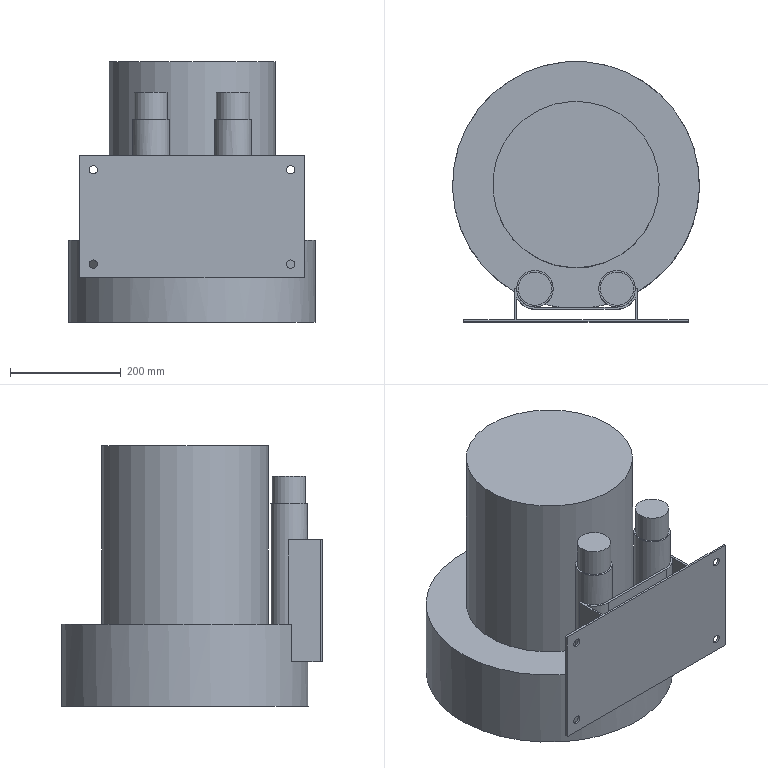Part | STEP file | High-pressure fan RB-81D-2  5.5 | 1 solid | 39 faces | box 445 x 470 x 470 mm | volume 48196616 mm3 | plane 25 | cylinder 14 | commonest cylinder face diameters 15 x4 66 x4 60 x2 74 x2 300 x1 445 x1
STEP:
#1=CARTESIAN_POINT('',(-107.,-187.5,300.));
#2=VERTEX_POINT('',#1);
#3=CARTESIAN_POINT('',(-74.,-220.5,300.));
#4=VERTEX_POINT('',#3);
#5=CARTESIAN_POINT('',(-74.,-187.5,300.));
#6=DIRECTION('',(0.,0.,1.));
#7=DIRECTION('',(-1.,0.,0.));
#8=AXIS2_PLACEMENT_3D('',#5,#6,#7);
#9=CIRCLE('',#8,33.);
#10=EDGE_CURVE('',#2,#4,#9,.T.);
#11=ORIENTED_EDGE('',*,*,#10,.T.);
#12=CARTESIAN_POINT('',(-74.,-220.5,148.));
#13=VERTEX_POINT('',#12);
#14=CARTESIAN_POINT('',(-74.,-220.5,300.));
#15=DIRECTION('',(0.,0.,-1.));
#16=VECTOR('',#15,1000.);
#17=LINE('',#14,#16);
#18=EDGE_CURVE('',#4,#13,#17,.T.);
#19=ORIENTED_EDGE('',*,*,#18,.T.);
#20=CARTESIAN_POINT('',(-56.197,-215.286,148.));
#21=VERTEX_POINT('',#20);
#22=CARTESIAN_POINT('',(-74.,-187.5,148.));
#23=DIRECTION('',(0.,0.,1.));
#24=DIRECTION('',(1.,0.,0.));
#25=AXIS2_PLACEMENT_3D('',#22,#23,#24);
#26=CIRCLE('',#25,33.);
#27=EDGE_CURVE('',#13,#21,#26,.T.);
#28=ORIENTED_EDGE('',*,*,#27,.T.);
#29=CARTESIAN_POINT('',(-107.,-187.5,148.));
#30=VERTEX_POINT('',#29);
#31=CARTESIAN_POINT('',(-74.,-187.5,148.));
#32=DIRECTION('',(0.,0.,-1.));
#33=DIRECTION('',(1.,0.,0.));
#34=AXIS2_PLACEMENT_3D('',#31,#32,#33);
#35=CIRCLE('',#34,33.);
#36=EDGE_CURVE('',#30,#21,#35,.T.);
#37=ORIENTED_EDGE('',*,*,#36,.F.);
#38=CARTESIAN_POINT('',(-107.,-187.5,300.));
#39=DIRECTION('',(0.,0.,-1.));
#40=VECTOR('',#39,1000.);
#41=LINE('',#38,#40);
#42=EDGE_CURVE('',#2,#30,#41,.T.);
#43=ORIENTED_EDGE('',*,*,#42,.F.);
#44=EDGE_LOOP('',(#11,#19,#28,#37,#43));
#45=FACE_OUTER_BOUND('',#44,.T.);
#46=CARTESIAN_POINT('',(-41.,-187.5,365.));
#47=VERTEX_POINT('',#46);
#48=CARTESIAN_POINT('',(-74.,-187.5,365.));
#49=DIRECTION('',(0.,0.,1.));
#50=DIRECTION('',(1.,0.,0.));
#51=AXIS2_PLACEMENT_3D('',#48,#49,#50);
#52=CIRCLE('',#51,33.);
#53=EDGE_CURVE('',#47,#47,#52,.T.);
#54=ORIENTED_EDGE('',*,*,#53,.F.);
#55=EDGE_LOOP('',(#54));
#56=FACE_OUTER_BOUND('',#55,.T.);
#57=CARTESIAN_POINT('',(-74.,-187.5,415.));
#58=DIRECTION('',(0.,0.,-1.));
#59=DIRECTION('',(-1.,0.,0.));
#60=AXIS2_PLACEMENT_3D('',#57,#58,#59);
#61=CYLINDRICAL_SURFACE('',#60,33.);
#62=ADVANCED_FACE('',(#45,#56),#61,.T.);
#63=CARTESIAN_POINT('',(74.,-220.5,300.));
#64=VERTEX_POINT('',#63);
#65=CARTESIAN_POINT('',(107.,-187.5,300.));
#66=VERTEX_POINT('',#65);
#67=CARTESIAN_POINT('',(74.,-187.5,300.));
#68=DIRECTION('',(0.,0.,1.));
#69=DIRECTION('',(-1.,0.,0.));
#70=AXIS2_PLACEMENT_3D('',#67,#68,#69);
#71=CIRCLE('',#70,33.);
#72=EDGE_CURVE('',#64,#66,#71,.T.);
#73=ORIENTED_EDGE('',*,*,#72,.T.);
#74=CARTESIAN_POINT('',(107.,-187.5,148.));
#75=VERTEX_POINT('',#74);
#76=CARTESIAN_POINT('',(107.,-187.5,300.));
#77=DIRECTION('',(0.,0.,-1.));
#78=VECTOR('',#77,1000.);
#79=LINE('',#76,#78);
#80=EDGE_CURVE('',#66,#75,#79,.T.);
#81=ORIENTED_EDGE('',*,*,#80,.T.);
#82=CARTESIAN_POINT('',(56.197,-215.286,148.));
#83=VERTEX_POINT('',#82);
#84=CARTESIAN_POINT('',(74.,-187.5,148.));
#85=DIRECTION('',(0.,0.,-1.));
#86=DIRECTION('',(1.,0.,0.));
#87=AXIS2_PLACEMENT_3D('',#84,#85,#86);
#88=CIRCLE('',#87,33.);
#89=EDGE_CURVE('',#83,#75,#88,.T.);
#90=ORIENTED_EDGE('',*,*,#89,.F.);
#91=CARTESIAN_POINT('',(74.,-220.5,148.));
#92=VERTEX_POINT('',#91);
#93=CARTESIAN_POINT('',(74.,-187.5,148.));
#94=DIRECTION('',(0.,0.,1.));
#95=DIRECTION('',(1.,0.,0.));
#96=AXIS2_PLACEMENT_3D('',#93,#94,#95);
#97=CIRCLE('',#96,33.);
#98=EDGE_CURVE('',#83,#92,#97,.T.);
#99=ORIENTED_EDGE('',*,*,#98,.T.);
#100=CARTESIAN_POINT('',(74.,-220.5,300.));
#101=DIRECTION('',(0.,0.,-1.));
#102=VECTOR('',#101,1000.);
#103=LINE('',#100,#102);
#104=EDGE_CURVE('',#64,#92,#103,.T.);
#105=ORIENTED_EDGE('',*,*,#104,.F.);
#106=EDGE_LOOP('',(#73,#81,#90,#99,#105));
#107=FACE_OUTER_BOUND('',#106,.T.);
#108=CARTESIAN_POINT('',(107.,-187.5,365.));
#109=VERTEX_POINT('',#108);
#110=CARTESIAN_POINT('',(74.,-187.5,365.));
#111=DIRECTION('',(0.,0.,1.));
#112=DIRECTION('',(1.,0.,0.));
#113=AXIS2_PLACEMENT_3D('',#110,#111,#112);
#114=CIRCLE('',#113,33.);
#115=EDGE_CURVE('',#109,#109,#114,.T.);
#116=ORIENTED_EDGE('',*,*,#115,.F.);
#117=EDGE_LOOP('',(#116));
#118=FACE_OUTER_BOUND('',#117,.T.);
#119=CARTESIAN_POINT('',(74.,-187.5,415.));
#120=DIRECTION('',(0.,0.,-1.));
#121=DIRECTION('',(-1.,0.,0.));
#122=AXIS2_PLACEMENT_3D('',#119,#120,#121);
#123=CYLINDRICAL_SURFACE('',#122,33.);
#124=ADVANCED_FACE('',(#107,#118),#123,.T.);
#125=CARTESIAN_POINT('',(111.,-192.835,148.));
#126=VERTEX_POINT('',#125);
#127=CARTESIAN_POINT('',(-111.,-192.835,148.));
#128=VERTEX_POINT('',#127);
#129=CARTESIAN_POINT('',(0.,0.,148.));
#130=DIRECTION('',(0.,0.,1.));
#131=DIRECTION('',(1.,0.,0.));
#132=AXIS2_PLACEMENT_3D('',#129,#130,#131);
#133=CIRCLE('',#132,222.5);
#134=EDGE_CURVE('',#126,#128,#133,.T.);
#135=ORIENTED_EDGE('',*,*,#134,.F.);
#136=CARTESIAN_POINT('',(111.,-192.835,80.));
#137=VERTEX_POINT('',#136);
#138=CARTESIAN_POINT('',(111.,-192.835,148.));
#139=DIRECTION('',(0.,0.,-1.));
#140=VECTOR('',#139,1000.);
#141=LINE('',#138,#140);
#142=EDGE_CURVE('',#126,#137,#141,.T.);
#143=ORIENTED_EDGE('',*,*,#142,.T.);
#144=CARTESIAN_POINT('',(105.981,-195.638,80.));
#145=VERTEX_POINT('',#144);
#146=CARTESIAN_POINT('',(0.,0.,80.));
#147=DIRECTION('',(0.,0.,-1.));
#148=DIRECTION('',(-1.,0.,0.));
#149=AXIS2_PLACEMENT_3D('',#146,#147,#148);
#150=CIRCLE('',#149,222.5);
#151=EDGE_CURVE('',#137,#145,#150,.T.);
#152=ORIENTED_EDGE('',*,*,#151,.T.);
#153=CARTESIAN_POINT('',(105.981,-195.638,148.));
#154=VERTEX_POINT('',#153);
#155=CARTESIAN_POINT('',(105.981,-195.638,190.));
#156=DIRECTION('',(0.,0.,1.));
#157=VECTOR('',#156,1000.);
#158=LINE('',#155,#157);
#159=EDGE_CURVE('',#145,#154,#158,.T.);
#160=ORIENTED_EDGE('',*,*,#159,.T.);
#161=CARTESIAN_POINT('',(0.,0.,148.));
#162=DIRECTION('',(0.,0.,1.));
#163=DIRECTION('',(1.,0.,0.));
#164=AXIS2_PLACEMENT_3D('',#161,#162,#163);
#165=CIRCLE('',#164,222.5);
#166=EDGE_CURVE('',#83,#154,#165,.T.);
#167=ORIENTED_EDGE('',*,*,#166,.F.);
#168=CARTESIAN_POINT('',(29.766,-220.5,148.));
#169=VERTEX_POINT('',#168);
#170=CARTESIAN_POINT('',(0.,0.,148.));
#171=DIRECTION('',(0.,0.,1.));
#172=DIRECTION('',(1.,0.,0.));
#173=AXIS2_PLACEMENT_3D('',#170,#171,#172);
#174=CIRCLE('',#173,222.5);
#175=EDGE_CURVE('',#169,#83,#174,.T.);
#176=ORIENTED_EDGE('',*,*,#175,.F.);
#177=CARTESIAN_POINT('',(29.766,-220.5,80.));
#178=VERTEX_POINT('',#177);
#179=CARTESIAN_POINT('',(29.766,-220.5,148.));
#180=DIRECTION('',(0.,0.,-1.));
#181=VECTOR('',#180,1000.);
#182=LINE('',#179,#181);
#183=EDGE_CURVE('',#169,#178,#182,.T.);
#184=ORIENTED_EDGE('',*,*,#183,.T.);
#185=CARTESIAN_POINT('',(-29.766,-220.5,80.));
#186=VERTEX_POINT('',#185);
#187=CARTESIAN_POINT('',(0.,0.,80.));
#188=DIRECTION('',(0.,0.,-1.));
#189=DIRECTION('',(-1.,0.,0.));
#190=AXIS2_PLACEMENT_3D('',#187,#188,#189);
#191=CIRCLE('',#190,222.5);
#192=EDGE_CURVE('',#178,#186,#191,.T.);
#193=ORIENTED_EDGE('',*,*,#192,.T.);
#194=CARTESIAN_POINT('',(-29.766,-220.5,148.));
#195=VERTEX_POINT('',#194);
#196=CARTESIAN_POINT('',(-29.766,-220.5,148.));
#197=DIRECTION('',(0.,0.,1.));
#198=VECTOR('',#197,1000.);
#199=LINE('',#196,#198);
#200=EDGE_CURVE('',#186,#195,#199,.T.);
#201=ORIENTED_EDGE('',*,*,#200,.T.);
#202=CARTESIAN_POINT('',(0.,0.,148.));
#203=DIRECTION('',(0.,0.,1.));
#204=DIRECTION('',(1.,0.,0.));
#205=AXIS2_PLACEMENT_3D('',#202,#203,#204);
#206=CIRCLE('',#205,222.5);
#207=EDGE_CURVE('',#21,#195,#206,.T.);
#208=ORIENTED_EDGE('',*,*,#207,.F.);
#209=CARTESIAN_POINT('',(-105.981,-195.638,148.));
#210=VERTEX_POINT('',#209);
#211=CARTESIAN_POINT('',(0.,0.,148.));
#212=DIRECTION('',(0.,0.,1.));
#213=DIRECTION('',(1.,0.,0.));
#214=AXIS2_PLACEMENT_3D('',#211,#212,#213);
#215=CIRCLE('',#214,222.5);
#216=EDGE_CURVE('',#210,#21,#215,.T.);
#217=ORIENTED_EDGE('',*,*,#216,.F.);
#218=CARTESIAN_POINT('',(-105.981,-195.638,80.));
#219=VERTEX_POINT('',#218);
#220=CARTESIAN_POINT('',(-105.981,-195.638,190.));
#221=DIRECTION('',(0.,0.,-1.));
#222=VECTOR('',#221,1000.);
#223=LINE('',#220,#222);
#224=EDGE_CURVE('',#210,#219,#223,.T.);
#225=ORIENTED_EDGE('',*,*,#224,.T.);
#226=CARTESIAN_POINT('',(-111.,-192.835,80.));
#227=VERTEX_POINT('',#226);
#228=CARTESIAN_POINT('',(0.,0.,80.));
#229=DIRECTION('',(0.,0.,-1.));
#230=DIRECTION('',(-1.,0.,0.));
#231=AXIS2_PLACEMENT_3D('',#228,#229,#230);
#232=CIRCLE('',#231,222.5);
#233=EDGE_CURVE('',#219,#227,#232,.T.);
#234=ORIENTED_EDGE('',*,*,#233,.T.);
#235=CARTESIAN_POINT('',(-111.,-192.835,148.));
#236=DIRECTION('',(0.,0.,1.));
#237=VECTOR('',#236,1000.);
#238=LINE('',#235,#237);
#239=EDGE_CURVE('',#227,#128,#238,.T.);
#240=ORIENTED_EDGE('',*,*,#239,.T.);
#241=EDGE_LOOP('',(#135,#143,#152,#160,#167,#176,#184,#193,#201,#208,#217,#225,#234,#240));
#242=FACE_OUTER_BOUND('',#241,.T.);
#243=CARTESIAN_POINT('',(222.5,0.,0.));
#244=VERTEX_POINT('',#243);
#245=CARTESIAN_POINT('',(0.,0.,0.));
#246=DIRECTION('',(0.,0.,1.));
#247=DIRECTION('',(1.,0.,0.));
#248=AXIS2_PLACEMENT_3D('',#245,#246,#247);
#249=CIRCLE('',#248,222.5);
#250=EDGE_CURVE('',#244,#244,#249,.T.);
#251=ORIENTED_EDGE('',*,*,#250,.T.);
#252=EDGE_LOOP('',(#251));
#253=FACE_OUTER_BOUND('',#252,.T.);
#254=CARTESIAN_POINT('',(0.,0.,148.));
#255=DIRECTION('',(0.,0.,-1.));
#256=DIRECTION('',(-1.,0.,0.));
#257=AXIS2_PLACEMENT_3D('',#254,#255,#256);
#258=CYLINDRICAL_SURFACE('',#257,222.5);
#259=ADVANCED_FACE('',(#242,#253),#258,.T.);
#260=CARTESIAN_POINT('',(111.,-187.5,148.));
#261=VERTEX_POINT('',#260);
#262=CARTESIAN_POINT('',(111.,0.,148.));
#263=DIRECTION('',(0.,1.,0.));
#264=VECTOR('',#263,1000.);
#265=LINE('',#262,#264);
#266=EDGE_CURVE('',#126,#261,#265,.T.);
#267=ORIENTED_EDGE('',*,*,#266,.F.);
#268=ORIENTED_EDGE('',*,*,#134,.T.);
#269=CARTESIAN_POINT('',(-111.,-187.5,148.));
#270=VERTEX_POINT('',#269);
#271=CARTESIAN_POINT('',(-111.,0.,148.));
#272=DIRECTION('',(0.,-1.,0.));
#273=VECTOR('',#272,1000.);
#274=LINE('',#271,#273);
#275=EDGE_CURVE('',#270,#128,#274,.T.);
#276=ORIENTED_EDGE('',*,*,#275,.F.);
#277=CARTESIAN_POINT('',(0.,-187.5,148.));
#278=DIRECTION('',(-1.,0.,0.));
#279=VECTOR('',#278,1000.);
#280=LINE('',#277,#279);
#281=EDGE_CURVE('',#30,#270,#280,.T.);
#282=ORIENTED_EDGE('',*,*,#281,.F.);
#283=ORIENTED_EDGE('',*,*,#36,.T.);
#284=ORIENTED_EDGE('',*,*,#207,.T.);
#285=CARTESIAN_POINT('',(0.,-220.5,148.));
#286=DIRECTION('',(-1.,0.,0.));
#287=VECTOR('',#286,1000.);
#288=LINE('',#285,#287);
#289=EDGE_CURVE('',#169,#195,#288,.T.);
#290=ORIENTED_EDGE('',*,*,#289,.F.);
#291=ORIENTED_EDGE('',*,*,#175,.T.);
#292=ORIENTED_EDGE('',*,*,#89,.T.);
#293=CARTESIAN_POINT('',(0.,-187.5,148.));
#294=DIRECTION('',(-1.,0.,0.));
#295=VECTOR('',#294,1000.);
#296=LINE('',#293,#295);
#297=EDGE_CURVE('',#261,#75,#296,.T.);
#298=ORIENTED_EDGE('',*,*,#297,.F.);
#299=EDGE_LOOP('',(#267,#268,#276,#282,#283,#284,#290,#291,#292,#298));
#300=FACE_OUTER_BOUND('',#299,.T.);
#301=CARTESIAN_POINT('',(150.,0.,148.));
#302=VERTEX_POINT('',#301);
#303=CARTESIAN_POINT('',(0.,0.,148.));
#304=DIRECTION('',(0.,0.,1.));
#305=DIRECTION('',(1.,0.,0.));
#306=AXIS2_PLACEMENT_3D('',#303,#304,#305);
#307=CIRCLE('',#306,150.);
#308=EDGE_CURVE('',#302,#302,#307,.T.);
#309=ORIENTED_EDGE('',*,*,#308,.F.);
#310=EDGE_LOOP('',(#309));
#311=FACE_BOUND('',#310,.T.);
#312=CARTESIAN_POINT('',(0.,0.,148.));
#313=DIRECTION('',(0.,0.,1.));
#314=DIRECTION('',(1.,0.,0.));
#315=AXIS2_PLACEMENT_3D('',#312,#313,#314);
#316=PLANE('',#315);
#317=ADVANCED_FACE('',(#300,#311),#316,.T.);
#318=ORIENTED_EDGE('',*,*,#250,.F.);
#319=EDGE_LOOP('',(#318));
#320=FACE_OUTER_BOUND('',#319,.T.);
#321=CARTESIAN_POINT('',(0.,0.,0.));
#322=DIRECTION('',(0.,0.,1.));
#323=DIRECTION('',(1.,0.,0.));
#324=AXIS2_PLACEMENT_3D('',#321,#322,#323);
#325=PLANE('',#324);
#326=ADVANCED_FACE('',(#320),#325,.F.);
#327=CARTESIAN_POINT('',(150.,0.,470.));
#328=VERTEX_POINT('',#327);
#329=CARTESIAN_POINT('',(0.,0.,470.));
#330=DIRECTION('',(0.,0.,1.));
#331=DIRECTION('',(1.,0.,0.));
#332=AXIS2_PLACEMENT_3D('',#329,#330,#331);
#333=CIRCLE('',#332,150.);
#334=EDGE_CURVE('',#328,#328,#333,.T.);
#335=ORIENTED_EDGE('',*,*,#334,.F.);
#336=EDGE_LOOP('',(#335));
#337=FACE_OUTER_BOUND('',#336,.T.);
#338=ORIENTED_EDGE('',*,*,#308,.T.);
#339=EDGE_LOOP('',(#338));
#340=FACE_OUTER_BOUND('',#339,.T.);
#341=CARTESIAN_POINT('',(0.,0.,470.));
#342=DIRECTION('',(0.,0.,-1.));
#343=DIRECTION('',(-1.,0.,0.));
#344=AXIS2_PLACEMENT_3D('',#341,#342,#343);
#345=CYLINDRICAL_SURFACE('',#344,150.);
#346=ADVANCED_FACE('',(#337,#340),#345,.T.);
#347=ORIENTED_EDGE('',*,*,#334,.T.);
#348=EDGE_LOOP('',(#347));
#349=FACE_OUTER_BOUND('',#348,.T.);
#350=CARTESIAN_POINT('',(0.,0.,470.));
#351=DIRECTION('',(0.,0.,1.));
#352=DIRECTION('',(1.,0.,0.));
#353=AXIS2_PLACEMENT_3D('',#350,#351,#352);
#354=PLANE('',#353);
#355=ADVANCED_FACE('',(#349),#354,.T.);
#356=CARTESIAN_POINT('',(-74.,-187.5,148.));
#357=DIRECTION('',(0.,0.,1.));
#358=DIRECTION('',(1.,0.,0.));
#359=AXIS2_PLACEMENT_3D('',#356,#357,#358);
#360=CIRCLE('',#359,33.);
#361=EDGE_CURVE('',#210,#13,#360,.T.);
#362=ORIENTED_EDGE('',*,*,#361,.F.);
#363=ORIENTED_EDGE('',*,*,#216,.T.);
#364=ORIENTED_EDGE('',*,*,#27,.F.);
#365=EDGE_LOOP('',(#362,#363,#364));
#366=FACE_OUTER_BOUND('',#365,.T.);
#367=CARTESIAN_POINT('',(-74.,-187.5,148.));
#368=DIRECTION('',(0.,0.,1.));
#369=DIRECTION('',(1.,0.,0.));
#370=AXIS2_PLACEMENT_3D('',#367,#368,#369);
#371=PLANE('',#370);
#372=ADVANCED_FACE('',(#366),#371,.F.);
#373=ORIENTED_EDGE('',*,*,#98,.F.);
#374=ORIENTED_EDGE('',*,*,#166,.T.);
#375=CARTESIAN_POINT('',(74.,-187.5,148.));
#376=DIRECTION('',(0.,0.,1.));
#377=DIRECTION('',(1.,0.,0.));
#378=AXIS2_PLACEMENT_3D('',#375,#376,#377);
#379=CIRCLE('',#378,33.);
#380=EDGE_CURVE('',#92,#154,#379,.T.);
#381=ORIENTED_EDGE('',*,*,#380,.F.);
#382=EDGE_LOOP('',(#373,#374,#381));
#383=FACE_OUTER_BOUND('',#382,.T.);
#384=CARTESIAN_POINT('',(74.,-187.5,148.));
#385=DIRECTION('',(0.,0.,1.));
#386=DIRECTION('',(1.,0.,0.));
#387=AXIS2_PLACEMENT_3D('',#384,#385,#386);
#388=PLANE('',#387);
#389=ADVANCED_FACE('',(#383),#388,.F.);
#390=ORIENTED_EDGE('',*,*,#142,.F.);
#391=ORIENTED_EDGE('',*,*,#266,.T.);
#392=CARTESIAN_POINT('',(111.,-187.5,300.));
#393=VERTEX_POINT('',#392);
#394=CARTESIAN_POINT('',(111.,-187.5,300.));
#395=DIRECTION('',(0.,0.,-1.));
#396=VECTOR('',#395,1000.);
#397=LINE('',#394,#396);
#398=EDGE_CURVE('',#393,#261,#397,.T.);
#399=ORIENTED_EDGE('',*,*,#398,.F.);
#400=CARTESIAN_POINT('',(111.,-243.5,300.));
#401=VERTEX_POINT('',#400);
#402=CARTESIAN_POINT('',(111.,-187.5,300.));
#403=DIRECTION('',(0.,-1.,0.));
#404=VECTOR('',#403,1000.);
#405=LINE('',#402,#404);
#406=EDGE_CURVE('',#393,#401,#405,.T.);
#407=ORIENTED_EDGE('',*,*,#406,.T.);
#408=CARTESIAN_POINT('',(111.,-243.5,80.));
#409=VERTEX_POINT('',#408);
#410=CARTESIAN_POINT('',(111.,-243.5,300.));
#411=DIRECTION('',(0.,0.,-1.));
#412=VECTOR('',#411,1000.);
#413=LINE('',#410,#412);
#414=EDGE_CURVE('',#401,#409,#413,.T.);
#415=ORIENTED_EDGE('',*,*,#414,.T.);
#416=CARTESIAN_POINT('',(111.,-187.5,80.));
#417=DIRECTION('',(0.,-1.,0.));
#418=VECTOR('',#417,1000.);
#419=LINE('',#416,#418);
#420=EDGE_CURVE('',#137,#409,#419,.T.);
#421=ORIENTED_EDGE('',*,*,#420,.F.);
#422=EDGE_LOOP('',(#390,#391,#399,#407,#415,#421));
#423=FACE_OUTER_BOUND('',#422,.T.);
#424=CARTESIAN_POINT('',(111.,-187.5,300.));
#425=DIRECTION('',(1.,0.,0.));
#426=DIRECTION('',(0.,1.,0.));
#427=AXIS2_PLACEMENT_3D('',#424,#425,#426);
#428=PLANE('',#427);
#429=ADVANCED_FACE('',(#423),#428,.T.);
#430=ORIENTED_EDGE('',*,*,#239,.F.);
#431=CARTESIAN_POINT('',(-111.,-243.5,80.));
#432=VERTEX_POINT('',#431);
#433=CARTESIAN_POINT('',(-111.,-187.5,80.));
#434=DIRECTION('',(0.,1.,0.));
#435=VECTOR('',#434,1000.);
#436=LINE('',#433,#435);
#437=EDGE_CURVE('',#432,#227,#436,.T.);
#438=ORIENTED_EDGE('',*,*,#437,.F.);
#439=CARTESIAN_POINT('',(-111.,-243.5,300.));
#440=VERTEX_POINT('',#439);
#441=CARTESIAN_POINT('',(-111.,-243.5,300.));
#442=DIRECTION('',(0.,0.,-1.));
#443=VECTOR('',#442,1000.);
#444=LINE('',#441,#443);
#445=EDGE_CURVE('',#440,#432,#444,.T.);
#446=ORIENTED_EDGE('',*,*,#445,.F.);
#447=CARTESIAN_POINT('',(-111.,-187.5,300.));
#448=VERTEX_POINT('',#447);
#449=CARTESIAN_POINT('',(-111.,-187.5,300.));
#450=DIRECTION('',(0.,1.,0.));
#451=VECTOR('',#450,1000.);
#452=LINE('',#449,#451);
#453=EDGE_CURVE('',#440,#448,#452,.T.);
#454=ORIENTED_EDGE('',*,*,#453,.T.);
#455=CARTESIAN_POINT('',(-111.,-187.5,300.));
#456=DIRECTION('',(0.,0.,-1.));
#457=VECTOR('',#456,1000.);
#458=LINE('',#455,#457);
#459=EDGE_CURVE('',#448,#270,#458,.T.);
#460=ORIENTED_EDGE('',*,*,#459,.T.);
#461=ORIENTED_EDGE('',*,*,#275,.T.);
#462=EDGE_LOOP('',(#430,#438,#446,#454,#460,#461));
#463=FACE_OUTER_BOUND('',#462,.T.);
#464=CARTESIAN_POINT('',(-111.,-187.5,300.));
#465=DIRECTION('',(-1.,0.,0.));
#466=DIRECTION('',(0.,0.,1.));
#467=AXIS2_PLACEMENT_3D('',#464,#465,#466);
#468=PLANE('',#467);
#469=ADVANCED_FACE('',(#463),#468,.T.);
#470=ORIENTED_EDGE('',*,*,#224,.F.);
#471=ORIENTED_EDGE('',*,*,#361,.T.);
#472=CARTESIAN_POINT('',(-74.,-220.5,80.));
#473=VERTEX_POINT('',#472);
#474=CARTESIAN_POINT('',(-74.,-220.5,300.));
#475=DIRECTION('',(0.,0.,-1.));
#476=VECTOR('',#475,1000.);
#477=LINE('',#474,#476);
#478=EDGE_CURVE('',#13,#473,#477,.T.);
#479=ORIENTED_EDGE('',*,*,#478,.T.);
#480=CARTESIAN_POINT('',(-74.,-187.5,80.));
#481=DIRECTION('',(0.,0.,1.));
#482=DIRECTION('',(-1.,0.,0.));
#483=AXIS2_PLACEMENT_3D('',#480,#481,#482);
#484=CIRCLE('',#483,33.);
#485=EDGE_CURVE('',#219,#473,#484,.T.);
#486=ORIENTED_EDGE('',*,*,#485,.F.);
#487=EDGE_LOOP('',(#470,#471,#479,#486));
#488=FACE_OUTER_BOUND('',#487,.T.);
#489=CARTESIAN_POINT('',(-74.,-187.5,300.));
#490=DIRECTION('',(0.,0.,-1.));
#491=DIRECTION('',(-1.,0.,0.));
#492=AXIS2_PLACEMENT_3D('',#489,#490,#491);
#493=CYLINDRICAL_SURFACE('',#492,33.);
#494=ADVANCED_FACE('',(#488),#493,.F.);
#495=ORIENTED_EDGE('',*,*,#159,.F.);
#496=CARTESIAN_POINT('',(74.,-220.5,80.));
#497=VERTEX_POINT('',#496);
#498=CARTESIAN_POINT('',(74.,-187.5,80.));
#499=DIRECTION('',(0.,0.,1.));
#500=DIRECTION('',(-1.,0.,0.));
#501=AXIS2_PLACEMENT_3D('',#498,#499,#500);
#502=CIRCLE('',#501,33.);
#503=EDGE_CURVE('',#497,#145,#502,.T.);
#504=ORIENTED_EDGE('',*,*,#503,.F.);
#505=CARTESIAN_POINT('',(74.,-220.5,300.));
#506=DIRECTION('',(0.,0.,-1.));
#507=VECTOR('',#506,1000.);
#508=LINE('',#505,#507);
#509=EDGE_CURVE('',#92,#497,#508,.T.);
#510=ORIENTED_EDGE('',*,*,#509,.F.);
#511=ORIENTED_EDGE('',*,*,#380,.T.);
#512=EDGE_LOOP('',(#495,#504,#510,#511));
#513=FACE_OUTER_BOUND('',#512,.T.);
#514=CARTESIAN_POINT('',(74.,-187.5,300.));
#515=DIRECTION('',(0.,0.,-1.));
#516=DIRECTION('',(-1.,0.,0.));
#517=AXIS2_PLACEMENT_3D('',#514,#515,#516);
#518=CYLINDRICAL_SURFACE('',#517,33.);
#519=ADVANCED_FACE('',(#513),#518,.F.);
#520=ORIENTED_EDGE('',*,*,#183,.F.);
#521=ORIENTED_EDGE('',*,*,#289,.T.);
#522=ORIENTED_EDGE('',*,*,#200,.F.);
#523=CARTESIAN_POINT('',(-74.,-220.5,80.));
#524=DIRECTION('',(1.,0.,0.));
#525=VECTOR('',#524,1000.);
#526=LINE('',#523,#525);
#527=EDGE_CURVE('',#473,#186,#526,.T.);
#528=ORIENTED_EDGE('',*,*,#527,.F.);
#529=ORIENTED_EDGE('',*,*,#478,.F.);
#530=ORIENTED_EDGE('',*,*,#18,.F.);
#531=CARTESIAN_POINT('',(-74.,-220.5,300.));
#532=DIRECTION('',(1.,0.,0.));
#533=VECTOR('',#532,1000.);
#534=LINE('',#531,#533);
#535=EDGE_CURVE('',#4,#64,#534,.T.);
#536=ORIENTED_EDGE('',*,*,#535,.T.);
#537=ORIENTED_EDGE('',*,*,#104,.T.);
#538=ORIENTED_EDGE('',*,*,#509,.T.);
#539=CARTESIAN_POINT('',(-74.,-220.5,80.));
#540=DIRECTION('',(1.,0.,0.));
#541=VECTOR('',#540,1000.);
#542=LINE('',#539,#541);
#543=EDGE_CURVE('',#178,#497,#542,.T.);
#544=ORIENTED_EDGE('',*,*,#543,.F.);
#545=EDGE_LOOP('',(#520,#521,#522,#528,#529,#530,#536,#537,#538,#544));
#546=FACE_OUTER_BOUND('',#545,.T.);
#547=CARTESIAN_POINT('',(-74.,-220.5,300.));
#548=DIRECTION('',(0.,1.,0.));
#549=DIRECTION('',(-1.,0.,0.));
#550=AXIS2_PLACEMENT_3D('',#547,#548,#549);
#551=PLANE('',#550);
#552=ADVANCED_FACE('',(#546),#551,.T.);
#553=CARTESIAN_POINT('',(202.5,-243.5,80.));
#554=VERTEX_POINT('',#553);
#555=CARTESIAN_POINT('',(202.5,-247.5,80.));
#556=VERTEX_POINT('',#555);
#557=CARTESIAN_POINT('',(202.5,-247.5,80.));
#558=DIRECTION('',(0.,-1.,0.));
#559=VECTOR('',#558,1000.);
#560=LINE('',#557,#559);
#561=EDGE_CURVE('',#554,#556,#560,.T.);
#562=ORIENTED_EDGE('',*,*,#561,.F.);
#563=CARTESIAN_POINT('',(202.5,-243.5,300.));
#564=VERTEX_POINT('',#563);
#565=CARTESIAN_POINT('',(202.5,-243.5,300.));
#566=DIRECTION('',(0.,0.,-1.));
#567=VECTOR('',#566,1000.);
#568=LINE('',#565,#567);
#569=EDGE_CURVE('',#564,#554,#568,.T.);
#570=ORIENTED_EDGE('',*,*,#569,.F.);
#571=CARTESIAN_POINT('',(202.5,-247.5,300.));
#572=VERTEX_POINT('',#571);
#573=CARTESIAN_POINT('',(202.5,-247.5,300.));
#574=DIRECTION('',(0.,-1.,0.));
#575=VECTOR('',#574,1000.);
#576=LINE('',#573,#575);
#577=EDGE_CURVE('',#564,#572,#576,.T.);
#578=ORIENTED_EDGE('',*,*,#577,.T.);
#579=CARTESIAN_POINT('',(202.5,-247.5,300.));
#580=DIRECTION('',(0.,0.,-1.));
#581=VECTOR('',#580,1000.);
#582=LINE('',#579,#581);
#583=EDGE_CURVE('',#572,#556,#582,.T.);
#584=ORIENTED_EDGE('',*,*,#583,.T.);
#585=EDGE_LOOP('',(#562,#570,#578,#584));
#586=FACE_OUTER_BOUND('',#585,.T.);
#587=CARTESIAN_POINT('',(202.5,-247.5,300.));
#588=DIRECTION('',(1.,0.,0.));
#589=DIRECTION('',(0.,0.,-1.));
#590=AXIS2_PLACEMENT_3D('',#587,#588,#589);
#591=PLANE('',#590);
#592=ADVANCED_FACE('',(#586),#591,.T.);
#593=CARTESIAN_POINT('',(178.,-243.5,112.5));
#594=VERTEX_POINT('',#593);
#595=CARTESIAN_POINT('',(178.,-243.5,105.));
#596=DIRECTION('',(0.,1.,0.));
#597=DIRECTION('',(0.,0.,1.));
#598=AXIS2_PLACEMENT_3D('',#595,#596,#597);
#599=CIRCLE('',#598,7.5);
#600=EDGE_CURVE('',#594,#594,#599,.T.);
#601=ORIENTED_EDGE('',*,*,#600,.F.);
#602=EDGE_LOOP('',(#601));
#603=FACE_BOUND('',#602,.T.);
#604=CARTESIAN_POINT('',(178.,-243.5,282.5));
#605=VERTEX_POINT('',#604);
#606=CARTESIAN_POINT('',(178.,-243.5,275.));
#607=DIRECTION('',(0.,1.,0.));
#608=DIRECTION('',(0.,0.,1.));
#609=AXIS2_PLACEMENT_3D('',#606,#607,#608);
#610=CIRCLE('',#609,7.5);
#611=EDGE_CURVE('',#605,#605,#610,.T.);
#612=ORIENTED_EDGE('',*,*,#611,.F.);
#613=EDGE_LOOP('',(#612));
#614=FACE_BOUND('',#613,.T.);
#615=CARTESIAN_POINT('',(111.,-243.5,80.));
#616=DIRECTION('',(1.,0.,0.));
#617=VECTOR('',#616,1000.);
#618=LINE('',#615,#617);
#619=EDGE_CURVE('',#409,#554,#618,.T.);
#620=ORIENTED_EDGE('',*,*,#619,.F.);
#621=ORIENTED_EDGE('',*,*,#414,.F.);
#622=CARTESIAN_POINT('',(111.,-243.5,300.));
#623=DIRECTION('',(1.,0.,0.));
#624=VECTOR('',#623,1000.);
#625=LINE('',#622,#624);
#626=EDGE_CURVE('',#401,#564,#625,.T.);
#627=ORIENTED_EDGE('',*,*,#626,.T.);
#628=ORIENTED_EDGE('',*,*,#569,.T.);
#629=EDGE_LOOP('',(#620,#621,#627,#628));
#630=FACE_OUTER_BOUND('',#629,.T.);
#631=CARTESIAN_POINT('',(111.,-243.5,300.));
#632=DIRECTION('',(0.,1.,0.));
#633=DIRECTION('',(0.,0.,1.));
#634=AXIS2_PLACEMENT_3D('',#631,#632,#633);
#635=PLANE('',#634);
#636=ADVANCED_FACE('',(#603,#614,#630),#635,.T.);
#637=ORIENTED_EDGE('',*,*,#398,.T.);
#638=ORIENTED_EDGE('',*,*,#297,.T.);
#639=ORIENTED_EDGE('',*,*,#80,.F.);
#640=CARTESIAN_POINT('',(107.,-187.5,300.));
#641=DIRECTION('',(1.,0.,0.));
#642=VECTOR('',#641,1000.);
#643=LINE('',#640,#642);
#644=EDGE_CURVE('',#66,#393,#643,.T.);
#645=ORIENTED_EDGE('',*,*,#644,.T.);
#646=EDGE_LOOP('',(#637,#638,#639,#645));
#647=FACE_OUTER_BOUND('',#646,.T.);
#648=CARTESIAN_POINT('',(107.,-187.5,300.));
#649=DIRECTION('',(0.,1.,0.));
#650=DIRECTION('',(0.,0.,1.));
#651=AXIS2_PLACEMENT_3D('',#648,#649,#650);
#652=PLANE('',#651);
#653=ADVANCED_FACE('',(#647),#652,.T.);
#654=ORIENTED_EDGE('',*,*,#42,.T.);
#655=ORIENTED_EDGE('',*,*,#281,.T.);
#656=ORIENTED_EDGE('',*,*,#459,.F.);
#657=CARTESIAN_POINT('',(-111.,-187.5,300.));
#658=DIRECTION('',(1.,0.,0.));
#659=VECTOR('',#658,1000.);
#660=LINE('',#657,#659);
#661=EDGE_CURVE('',#448,#2,#660,.T.);
#662=ORIENTED_EDGE('',*,*,#661,.T.);
#663=EDGE_LOOP('',(#654,#655,#656,#662));
#664=FACE_OUTER_BOUND('',#663,.T.);
#665=CARTESIAN_POINT('',(-111.,-187.5,300.));
#666=DIRECTION('',(0.,1.,0.));
#667=DIRECTION('',(0.,0.,1.));
#668=AXIS2_PLACEMENT_3D('',#665,#666,#667);
#669=PLANE('',#668);
#670=ADVANCED_FACE('',(#664),#669,.T.);
#671=CARTESIAN_POINT('',(-178.,-243.5,282.5));
#672=VERTEX_POINT('',#671);
#673=CARTESIAN_POINT('',(-178.,-243.5,275.));
#674=DIRECTION('',(0.,1.,0.));
#675=DIRECTION('',(0.,0.,1.));
#676=AXIS2_PLACEMENT_3D('',#673,#674,#675);
#677=CIRCLE('',#676,7.5);
#678=EDGE_CURVE('',#672,#672,#677,.T.);
#679=ORIENTED_EDGE('',*,*,#678,.F.);
#680=EDGE_LOOP('',(#679));
#681=FACE_BOUND('',#680,.T.);
#682=CARTESIAN_POINT('',(-178.,-243.5,112.5));
#683=VERTEX_POINT('',#682);
#684=CARTESIAN_POINT('',(-178.,-243.5,105.));
#685=DIRECTION('',(0.,1.,0.));
#686=DIRECTION('',(0.,0.,1.));
#687=AXIS2_PLACEMENT_3D('',#684,#685,#686);
#688=CIRCLE('',#687,7.5);
#689=EDGE_CURVE('',#683,#683,#688,.T.);
#690=ORIENTED_EDGE('',*,*,#689,.F.);
#691=EDGE_LOOP('',(#690));
#692=FACE_BOUND('',#691,.T.);
#693=CARTESIAN_POINT('',(-202.5,-243.5,80.));
#694=VERTEX_POINT('',#693);
#695=CARTESIAN_POINT('',(-202.5,-243.5,80.));
#696=DIRECTION('',(1.,0.,0.));
#697=VECTOR('',#696,1000.);
#698=LINE('',#695,#697);
#699=EDGE_CURVE('',#694,#432,#698,.T.);
#700=ORIENTED_EDGE('',*,*,#699,.F.);
#701=CARTESIAN_POINT('',(-202.5,-243.5,300.));
#702=VERTEX_POINT('',#701);
#703=CARTESIAN_POINT('',(-202.5,-243.5,300.));
#704=DIRECTION('',(0.,0.,-1.));
#705=VECTOR('',#704,1000.);
#706=LINE('',#703,#705);
#707=EDGE_CURVE('',#702,#694,#706,.T.);
#708=ORIENTED_EDGE('',*,*,#707,.F.);
#709=CARTESIAN_POINT('',(-202.5,-243.5,300.));
#710=DIRECTION('',(1.,0.,0.));
#711=VECTOR('',#710,1000.);
#712=LINE('',#709,#711);
#713=EDGE_CURVE('',#702,#440,#712,.T.);
#714=ORIENTED_EDGE('',*,*,#713,.T.);
#715=ORIENTED_EDGE('',*,*,#445,.T.);
#716=EDGE_LOOP('',(#700,#708,#714,#715));
#717=FACE_OUTER_BOUND('',#716,.T.);
#718=CARTESIAN_POINT('',(-202.5,-243.5,300.));
#719=DIRECTION('',(0.,1.,0.));
#720=DIRECTION('',(0.,0.,1.));
#721=AXIS2_PLACEMENT_3D('',#718,#719,#720);
#722=PLANE('',#721);
#723=ADVANCED_FACE('',(#681,#692,#717),#722,.T.);
#724=CARTESIAN_POINT('',(-202.5,-247.5,80.));
#725=VERTEX_POINT('',#724);
#726=CARTESIAN_POINT('',(-202.5,-243.5,80.));
#727=DIRECTION('',(0.,1.,0.));
#728=VECTOR('',#727,1000.);
#729=LINE('',#726,#728);
#730=EDGE_CURVE('',#725,#694,#729,.T.);
#731=ORIENTED_EDGE('',*,*,#730,.F.);
#732=CARTESIAN_POINT('',(-202.5,-247.5,300.));
#733=VERTEX_POINT('',#732);
#734=CARTESIAN_POINT('',(-202.5,-247.5,300.));
#735=DIRECTION('',(0.,0.,-1.));
#736=VECTOR('',#735,1000.);
#737=LINE('',#734,#736);
#738=EDGE_CURVE('',#733,#725,#737,.T.);
#739=ORIENTED_EDGE('',*,*,#738,.F.);
#740=CARTESIAN_POINT('',(-202.5,-243.5,300.));
#741=DIRECTION('',(0.,1.,0.));
#742=VECTOR('',#741,1000.);
#743=LINE('',#740,#742);
#744=EDGE_CURVE('',#733,#702,#743,.T.);
#745=ORIENTED_EDGE('',*,*,#744,.T.);
#746=ORIENTED_EDGE('',*,*,#707,.T.);
#747=EDGE_LOOP('',(#731,#739,#745,#746));
#748=FACE_OUTER_BOUND('',#747,.T.);
#749=CARTESIAN_POINT('',(-202.5,-243.5,300.));
#750=DIRECTION('',(-1.,0.,0.));
#751=DIRECTION('',(0.,0.,1.));
#752=AXIS2_PLACEMENT_3D('',#749,#750,#751);
#753=PLANE('',#752);
#754=ADVANCED_FACE('',(#748),#753,.T.);
#755=CARTESIAN_POINT('',(-178.,-247.5,282.5));
#756=VERTEX_POINT('',#755);
#757=CARTESIAN_POINT('',(-178.,-247.5,275.));
#758=DIRECTION('',(0.,1.,0.));
#759=DIRECTION('',(0.,0.,1.));
#760=AXIS2_PLACEMENT_3D('',#757,#758,#759);
#761=CIRCLE('',#760,7.5);
#762=EDGE_CURVE('',#756,#756,#761,.T.);
#763=ORIENTED_EDGE('',*,*,#762,.T.);
#764=EDGE_LOOP('',(#763));
#765=FACE_BOUND('',#764,.T.);
#766=CARTESIAN_POINT('',(178.,-247.5,112.5));
#767=VERTEX_POINT('',#766);
#768=CARTESIAN_POINT('',(178.,-247.5,105.));
#769=DIRECTION('',(0.,1.,0.));
#770=DIRECTION('',(0.,0.,1.));
#771=AXIS2_PLACEMENT_3D('',#768,#769,#770);
#772=CIRCLE('',#771,7.5);
#773=EDGE_CURVE('',#767,#767,#772,.T.);
#774=ORIENTED_EDGE('',*,*,#773,.T.);
#775=EDGE_LOOP('',(#774));
#776=FACE_BOUND('',#775,.T.);
#777=CARTESIAN_POINT('',(178.,-247.5,282.5));
#778=VERTEX_POINT('',#777);
#779=CARTESIAN_POINT('',(178.,-247.5,275.));
#780=DIRECTION('',(0.,1.,0.));
#781=DIRECTION('',(0.,0.,1.));
#782=AXIS2_PLACEMENT_3D('',#779,#780,#781);
#783=CIRCLE('',#782,7.5);
#784=EDGE_CURVE('',#778,#778,#783,.T.);
#785=ORIENTED_EDGE('',*,*,#784,.T.);
#786=EDGE_LOOP('',(#785));
#787=FACE_BOUND('',#786,.T.);
#788=CARTESIAN_POINT('',(-178.,-247.5,112.5));
#789=VERTEX_POINT('',#788);
#790=CARTESIAN_POINT('',(-178.,-247.5,105.));
#791=DIRECTION('',(0.,1.,0.));
#792=DIRECTION('',(0.,0.,1.));
#793=AXIS2_PLACEMENT_3D('',#790,#791,#792);
#794=CIRCLE('',#793,7.5);
#795=EDGE_CURVE('',#789,#789,#794,.T.);
#796=ORIENTED_EDGE('',*,*,#795,.T.);
#797=EDGE_LOOP('',(#796));
#798=FACE_BOUND('',#797,.T.);
#799=CARTESIAN_POINT('',(202.5,-247.5,80.));
#800=DIRECTION('',(-1.,0.,0.));
#801=VECTOR('',#800,1000.);
#802=LINE('',#799,#801);
#803=EDGE_CURVE('',#556,#725,#802,.T.);
#804=ORIENTED_EDGE('',*,*,#803,.F.);
#805=ORIENTED_EDGE('',*,*,#583,.F.);
#806=CARTESIAN_POINT('',(202.5,-247.5,300.));
#807=DIRECTION('',(-1.,0.,0.));
#808=VECTOR('',#807,1000.);
#809=LINE('',#806,#808);
#810=EDGE_CURVE('',#572,#733,#809,.T.);
#811=ORIENTED_EDGE('',*,*,#810,.T.);
#812=ORIENTED_EDGE('',*,*,#738,.T.);
#813=EDGE_LOOP('',(#804,#805,#811,#812));
#814=FACE_OUTER_BOUND('',#813,.T.);
#815=CARTESIAN_POINT('',(202.5,-247.5,300.));
#816=DIRECTION('',(0.,-1.,0.));
#817=DIRECTION('',(1.,0.,0.));
#818=AXIS2_PLACEMENT_3D('',#815,#816,#817);
#819=PLANE('',#818);
#820=ADVANCED_FACE('',(#765,#776,#787,#798,#814),#819,.T.);
#821=CARTESIAN_POINT('',(-74.,-224.5,300.));
#822=VERTEX_POINT('',#821);
#823=CARTESIAN_POINT('',(74.,-224.5,300.));
#824=VERTEX_POINT('',#823);
#825=CARTESIAN_POINT('',(-74.,-224.5,300.));
#826=DIRECTION('',(1.,0.,0.));
#827=VECTOR('',#826,1000.);
#828=LINE('',#825,#827);
#829=EDGE_CURVE('',#822,#824,#828,.T.);
#830=ORIENTED_EDGE('',*,*,#829,.T.);
#831=CARTESIAN_POINT('',(107.,-204.233,300.));
#832=VERTEX_POINT('',#831);
#833=CARTESIAN_POINT('',(74.,-187.5,300.));
#834=DIRECTION('',(0.,0.,1.));
#835=DIRECTION('',(-1.,0.,0.));
#836=AXIS2_PLACEMENT_3D('',#833,#834,#835);
#837=CIRCLE('',#836,37.);
#838=EDGE_CURVE('',#824,#832,#837,.T.);
#839=ORIENTED_EDGE('',*,*,#838,.T.);
#840=CARTESIAN_POINT('',(107.,-243.5,300.));
#841=VERTEX_POINT('',#840);
#842=CARTESIAN_POINT('',(107.,-204.233,300.));
#843=DIRECTION('',(0.,-1.,0.));
#844=VECTOR('',#843,1000.);
#845=LINE('',#842,#844);
#846=EDGE_CURVE('',#832,#841,#845,.T.);
#847=ORIENTED_EDGE('',*,*,#846,.T.);
#848=CARTESIAN_POINT('',(-107.,-243.5,300.));
#849=VERTEX_POINT('',#848);
#850=CARTESIAN_POINT('',(-107.,-243.5,300.));
#851=DIRECTION('',(-1.,0.,0.));
#852=VECTOR('',#851,1000.);
#853=LINE('',#850,#852);
#854=EDGE_CURVE('',#841,#849,#853,.T.);
#855=ORIENTED_EDGE('',*,*,#854,.T.);
#856=CARTESIAN_POINT('',(-107.,-204.233,300.));
#857=VERTEX_POINT('',#856);
#858=CARTESIAN_POINT('',(-107.,-204.233,300.));
#859=DIRECTION('',(0.,1.,0.));
#860=VECTOR('',#859,1000.);
#861=LINE('',#858,#860);
#862=EDGE_CURVE('',#849,#857,#861,.T.);
#863=ORIENTED_EDGE('',*,*,#862,.T.);
#864=CARTESIAN_POINT('',(-74.,-187.5,300.));
#865=DIRECTION('',(0.,0.,1.));
#866=DIRECTION('',(-1.,0.,0.));
#867=AXIS2_PLACEMENT_3D('',#864,#865,#866);
#868=CIRCLE('',#867,37.);
#869=EDGE_CURVE('',#857,#822,#868,.T.);
#870=ORIENTED_EDGE('',*,*,#869,.T.);
#871=EDGE_LOOP('',(#830,#839,#847,#855,#863,#870));
#872=FACE_BOUND('',#871,.T.);
#873=ORIENTED_EDGE('',*,*,#577,.F.);
#874=ORIENTED_EDGE('',*,*,#626,.F.);
#875=ORIENTED_EDGE('',*,*,#406,.F.);
#876=ORIENTED_EDGE('',*,*,#644,.F.);
#877=ORIENTED_EDGE('',*,*,#72,.F.);
#878=ORIENTED_EDGE('',*,*,#535,.F.);
#879=ORIENTED_EDGE('',*,*,#10,.F.);
#880=ORIENTED_EDGE('',*,*,#661,.F.);
#881=ORIENTED_EDGE('',*,*,#453,.F.);
#882=ORIENTED_EDGE('',*,*,#713,.F.);
#883=ORIENTED_EDGE('',*,*,#744,.F.);
#884=ORIENTED_EDGE('',*,*,#810,.F.);
#885=EDGE_LOOP('',(#873,#874,#875,#876,#877,#878,#879,#880,#881,#882,#883,#884));
#886=FACE_OUTER_BOUND('',#885,.T.);
#887=CARTESIAN_POINT('',(74.,-187.5,300.));
#888=DIRECTION('',(0.,0.,-1.));
#889=DIRECTION('',(-1.,0.,0.));
#890=AXIS2_PLACEMENT_3D('',#887,#888,#889);
#891=PLANE('',#890);
#892=ADVANCED_FACE('',(#872,#886),#891,.F.);
#893=ORIENTED_EDGE('',*,*,#151,.F.);
#894=ORIENTED_EDGE('',*,*,#420,.T.);
#895=ORIENTED_EDGE('',*,*,#619,.T.);
#896=ORIENTED_EDGE('',*,*,#561,.T.);
#897=ORIENTED_EDGE('',*,*,#803,.T.);
#898=ORIENTED_EDGE('',*,*,#730,.T.);
#899=ORIENTED_EDGE('',*,*,#699,.T.);
#900=ORIENTED_EDGE('',*,*,#437,.T.);
#901=ORIENTED_EDGE('',*,*,#233,.F.);
#902=ORIENTED_EDGE('',*,*,#485,.T.);
#903=ORIENTED_EDGE('',*,*,#527,.T.);
#904=ORIENTED_EDGE('',*,*,#192,.F.);
#905=ORIENTED_EDGE('',*,*,#543,.T.);
#906=ORIENTED_EDGE('',*,*,#503,.T.);
#907=EDGE_LOOP('',(#893,#894,#895,#896,#897,#898,#899,#900,#901,#902,#903,#904,#905,#906));
#908=FACE_OUTER_BOUND('',#907,.T.);
#909=CARTESIAN_POINT('',(74.,-224.5,80.));
#910=VERTEX_POINT('',#909);
#911=CARTESIAN_POINT('',(107.,-204.233,80.));
#912=VERTEX_POINT('',#911);
#913=CARTESIAN_POINT('',(74.,-187.5,80.));
#914=DIRECTION('',(0.,0.,1.));
#915=DIRECTION('',(-1.,0.,0.));
#916=AXIS2_PLACEMENT_3D('',#913,#914,#915);
#917=CIRCLE('',#916,37.);
#918=EDGE_CURVE('',#910,#912,#917,.T.);
#919=ORIENTED_EDGE('',*,*,#918,.F.);
#920=CARTESIAN_POINT('',(-74.,-224.5,80.));
#921=VERTEX_POINT('',#920);
#922=CARTESIAN_POINT('',(-74.,-224.5,80.));
#923=DIRECTION('',(1.,0.,0.));
#924=VECTOR('',#923,1000.);
#925=LINE('',#922,#924);
#926=EDGE_CURVE('',#921,#910,#925,.T.);
#927=ORIENTED_EDGE('',*,*,#926,.F.);
#928=CARTESIAN_POINT('',(-107.,-204.233,80.));
#929=VERTEX_POINT('',#928);
#930=CARTESIAN_POINT('',(-74.,-187.5,80.));
#931=DIRECTION('',(0.,0.,1.));
#932=DIRECTION('',(-1.,0.,0.));
#933=AXIS2_PLACEMENT_3D('',#930,#931,#932);
#934=CIRCLE('',#933,37.);
#935=EDGE_CURVE('',#929,#921,#934,.T.);
#936=ORIENTED_EDGE('',*,*,#935,.F.);
#937=CARTESIAN_POINT('',(-107.,-243.5,80.));
#938=VERTEX_POINT('',#937);
#939=CARTESIAN_POINT('',(-107.,-204.233,80.));
#940=DIRECTION('',(0.,1.,0.));
#941=VECTOR('',#940,1000.);
#942=LINE('',#939,#941);
#943=EDGE_CURVE('',#938,#929,#942,.T.);
#944=ORIENTED_EDGE('',*,*,#943,.F.);
#945=CARTESIAN_POINT('',(107.,-243.5,80.));
#946=VERTEX_POINT('',#945);
#947=CARTESIAN_POINT('',(-107.,-243.5,80.));
#948=DIRECTION('',(-1.,0.,0.));
#949=VECTOR('',#948,1000.);
#950=LINE('',#947,#949);
#951=EDGE_CURVE('',#946,#938,#950,.T.);
#952=ORIENTED_EDGE('',*,*,#951,.F.);
#953=CARTESIAN_POINT('',(107.,-204.233,80.));
#954=DIRECTION('',(0.,-1.,0.));
#955=VECTOR('',#954,1000.);
#956=LINE('',#953,#955);
#957=EDGE_CURVE('',#912,#946,#956,.T.);
#958=ORIENTED_EDGE('',*,*,#957,.F.);
#959=EDGE_LOOP('',(#919,#927,#936,#944,#952,#958));
#960=FACE_BOUND('',#959,.T.);
#961=CARTESIAN_POINT('',(74.,-187.5,80.));
#962=DIRECTION('',(0.,0.,-1.));
#963=DIRECTION('',(-1.,0.,0.));
#964=AXIS2_PLACEMENT_3D('',#961,#962,#963);
#965=PLANE('',#964);
#966=ADVANCED_FACE('',(#908,#960),#965,.T.);
#967=ORIENTED_EDGE('',*,*,#918,.T.);
#968=CARTESIAN_POINT('',(107.,-204.233,300.));
#969=DIRECTION('',(0.,0.,-1.));
#970=VECTOR('',#969,1000.);
#971=LINE('',#968,#970);
#972=EDGE_CURVE('',#832,#912,#971,.T.);
#973=ORIENTED_EDGE('',*,*,#972,.F.);
#974=ORIENTED_EDGE('',*,*,#838,.F.);
#975=CARTESIAN_POINT('',(74.,-224.5,300.));
#976=DIRECTION('',(0.,0.,-1.));
#977=VECTOR('',#976,1000.);
#978=LINE('',#975,#977);
#979=EDGE_CURVE('',#824,#910,#978,.T.);
#980=ORIENTED_EDGE('',*,*,#979,.T.);
#981=EDGE_LOOP('',(#967,#973,#974,#980));
#982=FACE_OUTER_BOUND('',#981,.T.);
#983=CARTESIAN_POINT('',(74.,-187.5,300.));
#984=DIRECTION('',(0.,0.,-1.));
#985=DIRECTION('',(-1.,0.,0.));
#986=AXIS2_PLACEMENT_3D('',#983,#984,#985);
#987=CYLINDRICAL_SURFACE('',#986,37.);
#988=ADVANCED_FACE('',(#982),#987,.T.);
#989=ORIENTED_EDGE('',*,*,#926,.T.);
#990=ORIENTED_EDGE('',*,*,#979,.F.);
#991=ORIENTED_EDGE('',*,*,#829,.F.);
#992=CARTESIAN_POINT('',(-74.,-224.5,300.));
#993=DIRECTION('',(0.,0.,-1.));
#994=VECTOR('',#993,1000.);
#995=LINE('',#992,#994);
#996=EDGE_CURVE('',#822,#921,#995,.T.);
#997=ORIENTED_EDGE('',*,*,#996,.T.);
#998=EDGE_LOOP('',(#989,#990,#991,#997));
#999=FACE_OUTER_BOUND('',#998,.T.);
#1000=CARTESIAN_POINT('',(-74.,-224.5,300.));
#1001=DIRECTION('',(0.,1.,0.));
#1002=DIRECTION('',(-1.,0.,0.));
#1003=AXIS2_PLACEMENT_3D('',#1000,#1001,#1002);
#1004=PLANE('',#1003);
#1005=ADVANCED_FACE('',(#999),#1004,.F.);
#1006=ORIENTED_EDGE('',*,*,#935,.T.);
#1007=ORIENTED_EDGE('',*,*,#996,.F.);
#1008=ORIENTED_EDGE('',*,*,#869,.F.);
#1009=CARTESIAN_POINT('',(-107.,-204.233,300.));
#1010=DIRECTION('',(0.,0.,-1.));
#1011=VECTOR('',#1010,1000.);
#1012=LINE('',#1009,#1011);
#1013=EDGE_CURVE('',#857,#929,#1012,.T.);
#1014=ORIENTED_EDGE('',*,*,#1013,.T.);
#1015=EDGE_LOOP('',(#1006,#1007,#1008,#1014));
#1016=FACE_OUTER_BOUND('',#1015,.T.);
#1017=CARTESIAN_POINT('',(-74.,-187.5,300.));
#1018=DIRECTION('',(0.,0.,-1.));
#1019=DIRECTION('',(-1.,0.,0.));
#1020=AXIS2_PLACEMENT_3D('',#1017,#1018,#1019);
#1021=CYLINDRICAL_SURFACE('',#1020,37.);
#1022=ADVANCED_FACE('',(#1016),#1021,.T.);
#1023=ORIENTED_EDGE('',*,*,#943,.T.);
#1024=ORIENTED_EDGE('',*,*,#1013,.F.);
#1025=ORIENTED_EDGE('',*,*,#862,.F.);
#1026=CARTESIAN_POINT('',(-107.,-243.5,300.));
#1027=DIRECTION('',(0.,0.,-1.));
#1028=VECTOR('',#1027,1000.);
#1029=LINE('',#1026,#1028);
#1030=EDGE_CURVE('',#849,#938,#1029,.T.);
#1031=ORIENTED_EDGE('',*,*,#1030,.T.);
#1032=EDGE_LOOP('',(#1023,#1024,#1025,#1031));
#1033=FACE_OUTER_BOUND('',#1032,.T.);
#1034=CARTESIAN_POINT('',(-107.,-204.233,300.));
#1035=DIRECTION('',(-1.,0.,0.));
#1036=DIRECTION('',(0.,-1.,0.));
#1037=AXIS2_PLACEMENT_3D('',#1034,#1035,#1036);
#1038=PLANE('',#1037);
#1039=ADVANCED_FACE('',(#1033),#1038,.F.);
#1040=ORIENTED_EDGE('',*,*,#951,.T.);
#1041=ORIENTED_EDGE('',*,*,#1030,.F.);
#1042=ORIENTED_EDGE('',*,*,#854,.F.);
#1043=CARTESIAN_POINT('',(107.,-243.5,300.));
#1044=DIRECTION('',(0.,0.,-1.));
#1045=VECTOR('',#1044,1000.);
#1046=LINE('',#1043,#1045);
#1047=EDGE_CURVE('',#841,#946,#1046,.T.);
#1048=ORIENTED_EDGE('',*,*,#1047,.T.);
#1049=EDGE_LOOP('',(#1040,#1041,#1042,#1048));
#1050=FACE_OUTER_BOUND('',#1049,.T.);
#1051=CARTESIAN_POINT('',(-107.,-243.5,300.));
#1052=DIRECTION('',(0.,-1.,0.));
#1053=DIRECTION('',(1.,0.,0.));
#1054=AXIS2_PLACEMENT_3D('',#1051,#1052,#1053);
#1055=PLANE('',#1054);
#1056=ADVANCED_FACE('',(#1050),#1055,.F.);
#1057=ORIENTED_EDGE('',*,*,#957,.T.);
#1058=ORIENTED_EDGE('',*,*,#1047,.F.);
#1059=ORIENTED_EDGE('',*,*,#846,.F.);
#1060=ORIENTED_EDGE('',*,*,#972,.T.);
#1061=EDGE_LOOP('',(#1057,#1058,#1059,#1060));
#1062=FACE_OUTER_BOUND('',#1061,.T.);
#1063=CARTESIAN_POINT('',(107.,-204.233,300.));
#1064=DIRECTION('',(1.,0.,0.));
#1065=DIRECTION('',(0.,1.,0.));
#1066=AXIS2_PLACEMENT_3D('',#1063,#1064,#1065);
#1067=PLANE('',#1066);
#1068=ADVANCED_FACE('',(#1062),#1067,.F.);
#1069=ORIENTED_EDGE('',*,*,#795,.F.);
#1070=EDGE_LOOP('',(#1069));
#1071=FACE_OUTER_BOUND('',#1070,.T.);
#1072=ORIENTED_EDGE('',*,*,#689,.T.);
#1073=EDGE_LOOP('',(#1072));
#1074=FACE_OUTER_BOUND('',#1073,.T.);
#1075=CARTESIAN_POINT('',(-178.,-247.5,105.));
#1076=DIRECTION('',(0.,1.,0.));
#1077=DIRECTION('',(0.,0.,1.));
#1078=AXIS2_PLACEMENT_3D('',#1075,#1076,#1077);
#1079=CYLINDRICAL_SURFACE('',#1078,7.5);
#1080=ADVANCED_FACE('',(#1071,#1074),#1079,.F.);
#1081=ORIENTED_EDGE('',*,*,#784,.F.);
#1082=EDGE_LOOP('',(#1081));
#1083=FACE_OUTER_BOUND('',#1082,.T.);
#1084=ORIENTED_EDGE('',*,*,#611,.T.);
#1085=EDGE_LOOP('',(#1084));
#1086=FACE_OUTER_BOUND('',#1085,.T.);
#1087=CARTESIAN_POINT('',(178.,-247.5,275.));
#1088=DIRECTION('',(0.,1.,0.));
#1089=DIRECTION('',(0.,0.,1.));
#1090=AXIS2_PLACEMENT_3D('',#1087,#1088,#1089);
#1091=CYLINDRICAL_SURFACE('',#1090,7.5);
#1092=ADVANCED_FACE('',(#1083,#1086),#1091,.F.);
#1093=ORIENTED_EDGE('',*,*,#773,.F.);
#1094=EDGE_LOOP('',(#1093));
#1095=FACE_OUTER_BOUND('',#1094,.T.);
#1096=ORIENTED_EDGE('',*,*,#600,.T.);
#1097=EDGE_LOOP('',(#1096));
#1098=FACE_OUTER_BOUND('',#1097,.T.);
#1099=CARTESIAN_POINT('',(178.,-247.5,105.));
#1100=DIRECTION('',(0.,1.,0.));
#1101=DIRECTION('',(0.,0.,1.));
#1102=AXIS2_PLACEMENT_3D('',#1099,#1100,#1101);
#1103=CYLINDRICAL_SURFACE('',#1102,7.5);
#1104=ADVANCED_FACE('',(#1095,#1098),#1103,.F.);
#1105=ORIENTED_EDGE('',*,*,#762,.F.);
#1106=EDGE_LOOP('',(#1105));
#1107=FACE_OUTER_BOUND('',#1106,.T.);
#1108=ORIENTED_EDGE('',*,*,#678,.T.);
#1109=EDGE_LOOP('',(#1108));
#1110=FACE_OUTER_BOUND('',#1109,.T.);
#1111=CARTESIAN_POINT('',(-178.,-247.5,275.));
#1112=DIRECTION('',(0.,1.,0.));
#1113=DIRECTION('',(0.,0.,1.));
#1114=AXIS2_PLACEMENT_3D('',#1111,#1112,#1113);
#1115=CYLINDRICAL_SURFACE('',#1114,7.5);
#1116=ADVANCED_FACE('',(#1107,#1110),#1115,.F.);
#1117=CARTESIAN_POINT('',(104.,-187.5,365.));
#1118=VERTEX_POINT('',#1117);
#1119=CARTESIAN_POINT('',(74.,-187.5,365.));
#1120=DIRECTION('',(0.,0.,1.));
#1121=DIRECTION('',(1.,0.,0.));
#1122=AXIS2_PLACEMENT_3D('',#1119,#1120,#1121);
#1123=CIRCLE('',#1122,30.);
#1124=EDGE_CURVE('',#1118,#1118,#1123,.T.);
#1125=ORIENTED_EDGE('',*,*,#1124,.F.);
#1126=EDGE_LOOP('',(#1125));
#1127=FACE_BOUND('',#1126,.T.);
#1128=ORIENTED_EDGE('',*,*,#115,.T.);
#1129=EDGE_LOOP('',(#1128));
#1130=FACE_OUTER_BOUND('',#1129,.T.);
#1131=CARTESIAN_POINT('',(74.,-187.5,365.));
#1132=DIRECTION('',(0.,0.,1.));
#1133=DIRECTION('',(1.,0.,0.));
#1134=AXIS2_PLACEMENT_3D('',#1131,#1132,#1133);
#1135=PLANE('',#1134);
#1136=ADVANCED_FACE('',(#1127,#1130),#1135,.T.);
#1137=ORIENTED_EDGE('',*,*,#1124,.T.);
#1138=EDGE_LOOP('',(#1137));
#1139=FACE_OUTER_BOUND('',#1138,.T.);
#1140=CARTESIAN_POINT('',(104.,-187.5,415.));
#1141=VERTEX_POINT('',#1140);
#1142=CARTESIAN_POINT('',(74.,-187.5,415.));
#1143=DIRECTION('',(0.,0.,1.));
#1144=DIRECTION('',(1.,0.,0.));
#1145=AXIS2_PLACEMENT_3D('',#1142,#1143,#1144);
#1146=CIRCLE('',#1145,30.);
#1147=EDGE_CURVE('',#1141,#1141,#1146,.T.);
#1148=ORIENTED_EDGE('',*,*,#1147,.F.);
#1149=EDGE_LOOP('',(#1148));
#1150=FACE_OUTER_BOUND('',#1149,.T.);
#1151=CARTESIAN_POINT('',(74.,-187.5,365.));
#1152=DIRECTION('',(0.,0.,1.));
#1153=DIRECTION('',(1.,0.,0.));
#1154=AXIS2_PLACEMENT_3D('',#1151,#1152,#1153);
#1155=CYLINDRICAL_SURFACE('',#1154,30.);
#1156=ADVANCED_FACE('',(#1139,#1150),#1155,.T.);
#1157=CARTESIAN_POINT('',(-44.,-187.5,365.));
#1158=VERTEX_POINT('',#1157);
#1159=CARTESIAN_POINT('',(-74.,-187.5,365.));
#1160=DIRECTION('',(0.,0.,1.));
#1161=DIRECTION('',(1.,0.,0.));
#1162=AXIS2_PLACEMENT_3D('',#1159,#1160,#1161);
#1163=CIRCLE('',#1162,30.);
#1164=EDGE_CURVE('',#1158,#1158,#1163,.T.);
#1165=ORIENTED_EDGE('',*,*,#1164,.F.);
#1166=EDGE_LOOP('',(#1165));
#1167=FACE_BOUND('',#1166,.T.);
#1168=ORIENTED_EDGE('',*,*,#53,.T.);
#1169=EDGE_LOOP('',(#1168));
#1170=FACE_OUTER_BOUND('',#1169,.T.);
#1171=CARTESIAN_POINT('',(-74.,-187.5,365.));
#1172=DIRECTION('',(0.,0.,1.));
#1173=DIRECTION('',(1.,0.,0.));
#1174=AXIS2_PLACEMENT_3D('',#1171,#1172,#1173);
#1175=PLANE('',#1174);
#1176=ADVANCED_FACE('',(#1167,#1170),#1175,.T.);
#1177=ORIENTED_EDGE('',*,*,#1164,.T.);
#1178=EDGE_LOOP('',(#1177));
#1179=FACE_OUTER_BOUND('',#1178,.T.);
#1180=CARTESIAN_POINT('',(-44.,-187.5,415.));
#1181=VERTEX_POINT('',#1180);
#1182=CARTESIAN_POINT('',(-74.,-187.5,415.));
#1183=DIRECTION('',(0.,0.,1.));
#1184=DIRECTION('',(1.,0.,0.));
#1185=AXIS2_PLACEMENT_3D('',#1182,#1183,#1184);
#1186=CIRCLE('',#1185,30.);
#1187=EDGE_CURVE('',#1181,#1181,#1186,.T.);
#1188=ORIENTED_EDGE('',*,*,#1187,.F.);
#1189=EDGE_LOOP('',(#1188));
#1190=FACE_OUTER_BOUND('',#1189,.T.);
#1191=CARTESIAN_POINT('',(-74.,-187.5,365.));
#1192=DIRECTION('',(0.,0.,1.));
#1193=DIRECTION('',(1.,0.,0.));
#1194=AXIS2_PLACEMENT_3D('',#1191,#1192,#1193);
#1195=CYLINDRICAL_SURFACE('',#1194,30.);
#1196=ADVANCED_FACE('',(#1179,#1190),#1195,.T.);
#1197=ORIENTED_EDGE('',*,*,#1147,.T.);
#1198=EDGE_LOOP('',(#1197));
#1199=FACE_OUTER_BOUND('',#1198,.T.);
#1200=CARTESIAN_POINT('',(74.,-187.5,415.));
#1201=DIRECTION('',(0.,0.,1.));
#1202=DIRECTION('',(1.,0.,0.));
#1203=AXIS2_PLACEMENT_3D('',#1200,#1201,#1202);
#1204=PLANE('',#1203);
#1205=ADVANCED_FACE('',(#1199),#1204,.T.);
#1206=ORIENTED_EDGE('',*,*,#1187,.T.);
#1207=EDGE_LOOP('',(#1206));
#1208=FACE_OUTER_BOUND('',#1207,.T.);
#1209=CARTESIAN_POINT('',(-74.,-187.5,415.));
#1210=DIRECTION('',(0.,0.,1.));
#1211=DIRECTION('',(1.,0.,0.));
#1212=AXIS2_PLACEMENT_3D('',#1209,#1210,#1211);
#1213=PLANE('',#1212);
#1214=ADVANCED_FACE('',(#1208),#1213,.T.);
#1215=CLOSED_SHELL('',(#62,#124,#259,#317,#326,#346,#355,#372,#389,#429,#469,#494,#519,#552,#592,#636,#653,#670,#723,#754,#820,#892,#966,#988,#1005,#1022,#1039,#1056,#1068,#1080,#1092,#1104,#1116,#1136,#1156,#1176,#1196,#1205,#1214));
#1216=MANIFOLD_SOLID_BREP('',#1215);
#1217=CARTESIAN_POINT('',(0.,0.,0.));
#1218=DIRECTION('',(0.,0.,1.));
#1219=DIRECTION('',(1.,0.,0.));
#1220=AXIS2_PLACEMENT_3D('',#1217,#1218,#1219);
#1221=(LENGTH_UNIT()NAMED_UNIT(*)SI_UNIT(.MILLI.,.METRE.));
#1222=UNCERTAINTY_MEASURE_WITH_UNIT(LENGTH_MEASURE(0.00001),#1221,'','');
#1223=(NAMED_UNIT(*)PLANE_ANGLE_UNIT()SI_UNIT($,.RADIAN.));
#1224=(NAMED_UNIT(*)SI_UNIT($,.STERADIAN.)SOLID_ANGLE_UNIT());
#1225=(GEOMETRIC_REPRESENTATION_CONTEXT(3)GLOBAL_UNCERTAINTY_ASSIGNED_CONTEXT((#1222))GLOBAL_UNIT_ASSIGNED_CONTEXT((#1221,#1223,#1224))REPRESENTATION_CONTEXT('',''));
#1226=ADVANCED_BREP_SHAPE_REPRESENTATION('',(#1216,#1220),#1225);